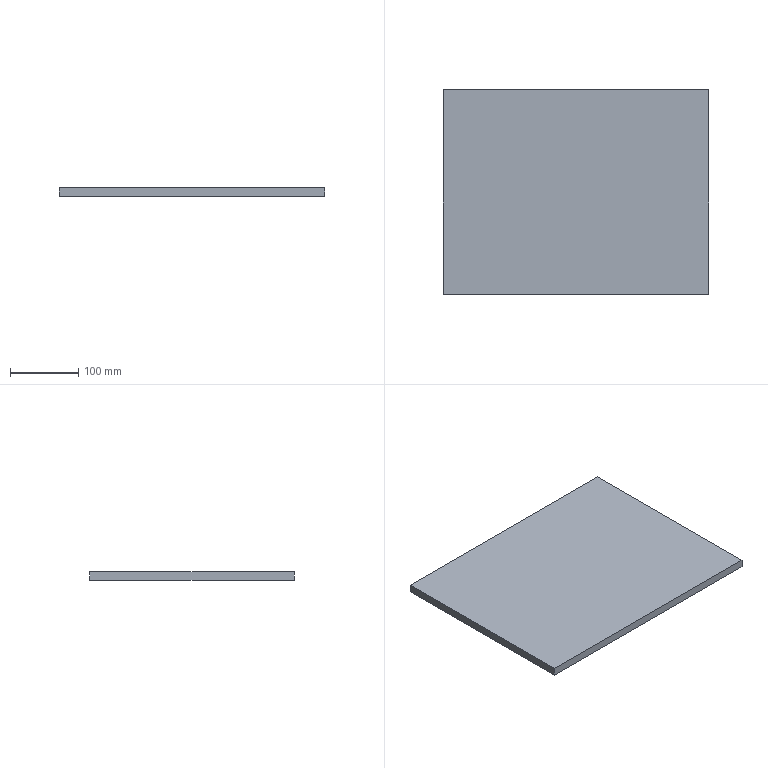Part | SolidWorks | features Extrusion 1 | 1 solid | 6 faces | box 390 x 300 x 12 mm | volume 1404000 mm3 | plane 6
STEP:
#1=CARTESIAN_POINT('',(0.,0.,0.));
#2=VERTEX_POINT('',#1);
#3=CARTESIAN_POINT('',(0.,-300.,0.));
#4=VERTEX_POINT('',#3);
#5=CARTESIAN_POINT('',(0.,0.,0.));
#6=DIRECTION('',(0.,-1.,0.));
#7=VECTOR('',#6,1000.);
#8=LINE('',#5,#7);
#9=EDGE_CURVE('',#2,#4,#8,.T.);
#10=ORIENTED_EDGE('',*,*,#9,.T.);
#11=CARTESIAN_POINT('',(0.,-300.,12.));
#12=VERTEX_POINT('',#11);
#13=CARTESIAN_POINT('',(0.,-300.,12.));
#14=DIRECTION('',(0.,0.,-1.));
#15=VECTOR('',#14,1000.);
#16=LINE('',#13,#15);
#17=EDGE_CURVE('',#12,#4,#16,.T.);
#18=ORIENTED_EDGE('',*,*,#17,.F.);
#19=CARTESIAN_POINT('',(0.,0.,12.));
#20=VERTEX_POINT('',#19);
#21=CARTESIAN_POINT('',(0.,0.,12.));
#22=DIRECTION('',(0.,-1.,0.));
#23=VECTOR('',#22,1000.);
#24=LINE('',#21,#23);
#25=EDGE_CURVE('',#20,#12,#24,.T.);
#26=ORIENTED_EDGE('',*,*,#25,.F.);
#27=CARTESIAN_POINT('',(0.,0.,12.));
#28=DIRECTION('',(0.,0.,-1.));
#29=VECTOR('',#28,1000.);
#30=LINE('',#27,#29);
#31=EDGE_CURVE('',#20,#2,#30,.T.);
#32=ORIENTED_EDGE('',*,*,#31,.T.);
#33=EDGE_LOOP('',(#10,#18,#26,#32));
#34=FACE_OUTER_BOUND('',#33,.T.);
#35=CARTESIAN_POINT('',(0.,0.,12.));
#36=DIRECTION('',(1.,0.,0.));
#37=DIRECTION('',(0.,1.,0.));
#38=AXIS2_PLACEMENT_3D('',#35,#36,#37);
#39=PLANE('',#38);
#40=ADVANCED_FACE('',(#34),#39,.F.);
#41=CARTESIAN_POINT('',(390.,-300.,0.));
#42=VERTEX_POINT('',#41);
#43=CARTESIAN_POINT('',(0.,-300.,0.));
#44=DIRECTION('',(1.,0.,0.));
#45=VECTOR('',#44,1000.);
#46=LINE('',#43,#45);
#47=EDGE_CURVE('',#4,#42,#46,.T.);
#48=ORIENTED_EDGE('',*,*,#47,.T.);
#49=CARTESIAN_POINT('',(390.,-300.,12.));
#50=VERTEX_POINT('',#49);
#51=CARTESIAN_POINT('',(390.,-300.,12.));
#52=DIRECTION('',(0.,0.,-1.));
#53=VECTOR('',#52,1000.);
#54=LINE('',#51,#53);
#55=EDGE_CURVE('',#50,#42,#54,.T.);
#56=ORIENTED_EDGE('',*,*,#55,.F.);
#57=CARTESIAN_POINT('',(0.,-300.,12.));
#58=DIRECTION('',(1.,0.,0.));
#59=VECTOR('',#58,1000.);
#60=LINE('',#57,#59);
#61=EDGE_CURVE('',#12,#50,#60,.T.);
#62=ORIENTED_EDGE('',*,*,#61,.F.);
#63=ORIENTED_EDGE('',*,*,#17,.T.);
#64=EDGE_LOOP('',(#48,#56,#62,#63));
#65=FACE_OUTER_BOUND('',#64,.T.);
#66=CARTESIAN_POINT('',(0.,-300.,12.));
#67=DIRECTION('',(0.,1.,0.));
#68=DIRECTION('',(0.,0.,1.));
#69=AXIS2_PLACEMENT_3D('',#66,#67,#68);
#70=PLANE('',#69);
#71=ADVANCED_FACE('',(#65),#70,.F.);
#72=CARTESIAN_POINT('',(390.,0.,0.));
#73=VERTEX_POINT('',#72);
#74=CARTESIAN_POINT('',(390.,0.,0.));
#75=DIRECTION('',(0.,1.,0.));
#76=VECTOR('',#75,1000.);
#77=LINE('',#74,#76);
#78=EDGE_CURVE('',#42,#73,#77,.T.);
#79=ORIENTED_EDGE('',*,*,#78,.T.);
#80=CARTESIAN_POINT('',(390.,0.,12.));
#81=VERTEX_POINT('',#80);
#82=CARTESIAN_POINT('',(390.,0.,12.));
#83=DIRECTION('',(0.,0.,-1.));
#84=VECTOR('',#83,1000.);
#85=LINE('',#82,#84);
#86=EDGE_CURVE('',#81,#73,#85,.T.);
#87=ORIENTED_EDGE('',*,*,#86,.F.);
#88=CARTESIAN_POINT('',(390.,0.,12.));
#89=DIRECTION('',(0.,1.,0.));
#90=VECTOR('',#89,1000.);
#91=LINE('',#88,#90);
#92=EDGE_CURVE('',#50,#81,#91,.T.);
#93=ORIENTED_EDGE('',*,*,#92,.F.);
#94=ORIENTED_EDGE('',*,*,#55,.T.);
#95=EDGE_LOOP('',(#79,#87,#93,#94));
#96=FACE_OUTER_BOUND('',#95,.T.);
#97=CARTESIAN_POINT('',(390.,0.,12.));
#98=DIRECTION('',(-1.,0.,0.));
#99=DIRECTION('',(0.,-1.,0.));
#100=AXIS2_PLACEMENT_3D('',#97,#98,#99);
#101=PLANE('',#100);
#102=ADVANCED_FACE('',(#96),#101,.F.);
#103=CARTESIAN_POINT('',(0.,0.,0.));
#104=DIRECTION('',(-1.,0.,0.));
#105=VECTOR('',#104,1000.);
#106=LINE('',#103,#105);
#107=EDGE_CURVE('',#73,#2,#106,.T.);
#108=ORIENTED_EDGE('',*,*,#107,.T.);
#109=ORIENTED_EDGE('',*,*,#31,.F.);
#110=CARTESIAN_POINT('',(0.,0.,12.));
#111=DIRECTION('',(-1.,0.,0.));
#112=VECTOR('',#111,1000.);
#113=LINE('',#110,#112);
#114=EDGE_CURVE('',#81,#20,#113,.T.);
#115=ORIENTED_EDGE('',*,*,#114,.F.);
#116=ORIENTED_EDGE('',*,*,#86,.T.);
#117=EDGE_LOOP('',(#108,#109,#115,#116));
#118=FACE_OUTER_BOUND('',#117,.T.);
#119=CARTESIAN_POINT('',(0.,0.,12.));
#120=DIRECTION('',(0.,-1.,0.));
#121=DIRECTION('',(0.,0.,-1.));
#122=AXIS2_PLACEMENT_3D('',#119,#120,#121);
#123=PLANE('',#122);
#124=ADVANCED_FACE('',(#118),#123,.F.);
#125=ORIENTED_EDGE('',*,*,#25,.T.);
#126=ORIENTED_EDGE('',*,*,#61,.T.);
#127=ORIENTED_EDGE('',*,*,#92,.T.);
#128=ORIENTED_EDGE('',*,*,#114,.T.);
#129=EDGE_LOOP('',(#125,#126,#127,#128));
#130=FACE_OUTER_BOUND('',#129,.T.);
#131=CARTESIAN_POINT('',(0.,0.,12.));
#132=DIRECTION('',(0.,0.,1.));
#133=DIRECTION('',(1.,0.,0.));
#134=AXIS2_PLACEMENT_3D('',#131,#132,#133);
#135=PLANE('',#134);
#136=ADVANCED_FACE('',(#130),#135,.T.);
#137=ORIENTED_EDGE('',*,*,#9,.F.);
#138=ORIENTED_EDGE('',*,*,#107,.F.);
#139=ORIENTED_EDGE('',*,*,#78,.F.);
#140=ORIENTED_EDGE('',*,*,#47,.F.);
#141=EDGE_LOOP('',(#137,#138,#139,#140));
#142=FACE_OUTER_BOUND('',#141,.T.);
#143=CARTESIAN_POINT('',(0.,0.,0.));
#144=DIRECTION('',(0.,0.,1.));
#145=DIRECTION('',(1.,0.,0.));
#146=AXIS2_PLACEMENT_3D('',#143,#144,#145);
#147=PLANE('',#146);
#148=ADVANCED_FACE('',(#142),#147,.F.);
#149=CLOSED_SHELL('',(#40,#71,#102,#124,#136,#148));
#150=MANIFOLD_SOLID_BREP('',#149);
#151=CARTESIAN_POINT('',(0.,0.,0.));
#152=DIRECTION('',(0.,0.,1.));
#153=DIRECTION('',(1.,0.,0.));
#154=AXIS2_PLACEMENT_3D('',#151,#152,#153);
#155=(LENGTH_UNIT()NAMED_UNIT(*)SI_UNIT(.MILLI.,.METRE.));
#156=UNCERTAINTY_MEASURE_WITH_UNIT(LENGTH_MEASURE(0.00001),#155,'','');
#157=(NAMED_UNIT(*)PLANE_ANGLE_UNIT()SI_UNIT($,.RADIAN.));
#158=(NAMED_UNIT(*)SI_UNIT($,.STERADIAN.)SOLID_ANGLE_UNIT());
#159=(GEOMETRIC_REPRESENTATION_CONTEXT(3)GLOBAL_UNCERTAINTY_ASSIGNED_CONTEXT((#156))GLOBAL_UNIT_ASSIGNED_CONTEXT((#155,#157,#158))REPRESENTATION_CONTEXT('',''));
#160=ADVANCED_BREP_SHAPE_REPRESENTATION('',(#150,#154),#159);